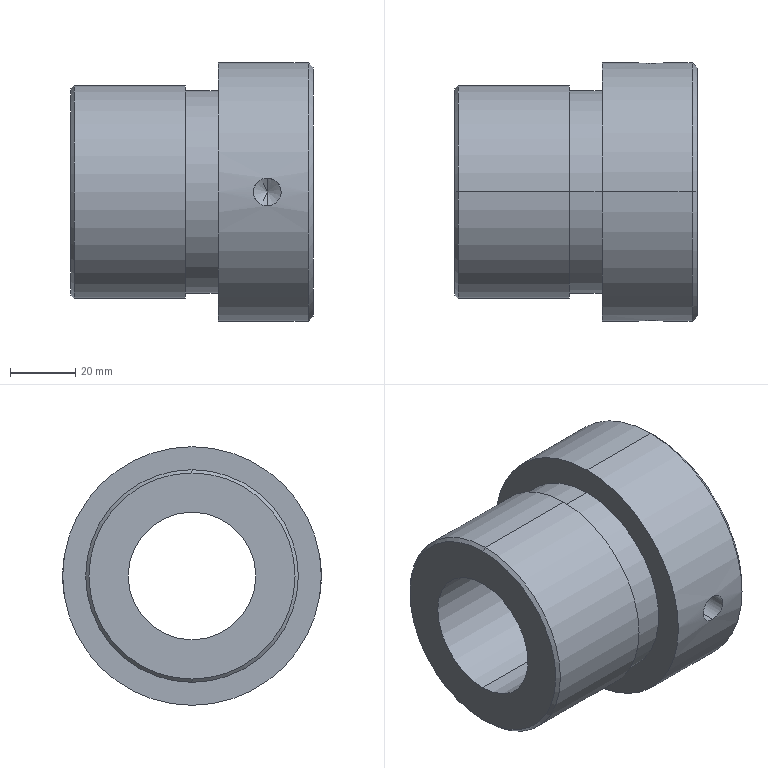Part | SolidWorks | features ICE 9, Chamfer 7, Draft 2, HoleWzd 2, Extrusion 1, Fillet 1, MirrorPattern 1, MoveFace 1 | 1 solid | 24 faces | box 74 x 79 x 79 mm | volume 198251 mm3 | cylinder 12 | cone 8 | plane 4 | commonest cylinder face diameters 8.5 x4 39 x2 62 x2 65 x2 79 x2
STEP:
#1=CARTESIAN_POINT('',(0.,0.,19.5));
#2=VERTEX_POINT('',#1);
#3=CARTESIAN_POINT('',(0.,0.,-19.5));
#4=VERTEX_POINT('',#3);
#5=CARTESIAN_POINT('',(0.,0.,0.));
#6=DIRECTION('',(1.,0.,0.));
#7=DIRECTION('',(0.,0.,-1.));
#8=AXIS2_PLACEMENT_3D('',#5,#6,#7);
#9=CIRCLE('',#8,19.5);
#10=EDGE_CURVE('',#2,#4,#9,.T.);
#11=ORIENTED_EDGE('',*,*,#10,.F.);
#12=CARTESIAN_POINT('',(74.,0.,19.5));
#13=VERTEX_POINT('',#12);
#14=CARTESIAN_POINT('',(74.,0.,19.5));
#15=DIRECTION('',(1.,0.,0.));
#16=VECTOR('',#15,1000.);
#17=LINE('',#14,#16);
#18=EDGE_CURVE('',#2,#13,#17,.T.);
#19=ORIENTED_EDGE('',*,*,#18,.T.);
#20=CARTESIAN_POINT('',(74.,0.,-19.5));
#21=VERTEX_POINT('',#20);
#22=CARTESIAN_POINT('',(74.,0.,0.));
#23=DIRECTION('',(1.,0.,0.));
#24=DIRECTION('',(0.,0.,-1.));
#25=AXIS2_PLACEMENT_3D('',#22,#23,#24);
#26=CIRCLE('',#25,19.5);
#27=EDGE_CURVE('',#13,#21,#26,.T.);
#28=ORIENTED_EDGE('',*,*,#27,.T.);
#29=CARTESIAN_POINT('',(74.,0.,-19.5));
#30=DIRECTION('',(1.,0.,0.));
#31=VECTOR('',#30,1000.);
#32=LINE('',#29,#31);
#33=EDGE_CURVE('',#4,#21,#32,.T.);
#34=ORIENTED_EDGE('',*,*,#33,.F.);
#35=EDGE_LOOP('',(#11,#19,#28,#34));
#36=FACE_OUTER_BOUND('',#35,.T.);
#37=CARTESIAN_POINT('',(74.,0.,0.));
#38=DIRECTION('',(1.,0.,0.));
#39=DIRECTION('',(0.,0.,-1.));
#40=AXIS2_PLACEMENT_3D('',#37,#38,#39);
#41=CYLINDRICAL_SURFACE('',#40,19.5);
#42=ADVANCED_FACE('',(#36),#41,.F.);
#43=CARTESIAN_POINT('',(60.,24.946,0.));
#44=VERTEX_POINT('',#43);
#45=CARTESIAN_POINT('',(60.,27.5,4.25));
#46=VERTEX_POINT('',#45);
#47=CARTESIAN_POINT('',(60.,27.5,4.25));
#48=DIRECTION('',(0.,0.515,0.8572));
#49=VECTOR('',#48,1000.);
#50=LINE('',#47,#49);
#51=EDGE_CURVE('',#44,#46,#50,.T.);
#52=ORIENTED_EDGE('',*,*,#51,.F.);
#53=CARTESIAN_POINT('',(60.,27.5,-4.25));
#54=VERTEX_POINT('',#53);
#55=CARTESIAN_POINT('',(60.,27.5,-4.25));
#56=DIRECTION('',(0.,0.515,-0.8572));
#57=VECTOR('',#56,1000.);
#58=LINE('',#55,#57);
#59=EDGE_CURVE('',#44,#54,#58,.T.);
#60=ORIENTED_EDGE('',*,*,#59,.T.);
#61=CARTESIAN_POINT('',(60.,27.5,0.));
#62=DIRECTION('',(0.,1.,0.));
#63=DIRECTION('',(0.,0.,1.));
#64=AXIS2_PLACEMENT_3D('',#61,#62,#63);
#65=CIRCLE('',#64,4.25);
#66=EDGE_CURVE('',#54,#46,#65,.T.);
#67=ORIENTED_EDGE('',*,*,#66,.T.);
#68=EDGE_LOOP('',(#52,#60,#67));
#69=FACE_OUTER_BOUND('',#68,.T.);
#70=CARTESIAN_POINT('',(60.,27.5,0.));
#71=DIRECTION('',(0.,1.,0.));
#72=DIRECTION('',(0.,0.,1.));
#73=AXIS2_PLACEMENT_3D('',#70,#71,#72);
#74=CONICAL_SURFACE('',#73,4.25,1.03);
#75=ADVANCED_FACE('',(#69),#74,.F.);
#76=ORIENTED_EDGE('',*,*,#66,.F.);
#77=CARTESIAN_POINT('',(60.,39.271,-4.25));
#78=VERTEX_POINT('',#77);
#79=CARTESIAN_POINT('',(60.,37.5,-4.25));
#80=DIRECTION('',(0.,1.,0.));
#81=VECTOR('',#80,1000.);
#82=LINE('',#79,#81);
#83=EDGE_CURVE('',#54,#78,#82,.T.);
#84=ORIENTED_EDGE('',*,*,#83,.T.);
#85=CARTESIAN_POINT('',(60.,39.271,4.25));
#86=VERTEX_POINT('',#85);
#87=CARTESIAN_POINT('',(60.,39.271,-4.25));
#88=CARTESIAN_POINT('',(59.723,39.271,-4.25));
#89=CARTESIAN_POINT('',(59.447,39.274,-4.223));
#90=CARTESIAN_POINT('',(58.898,39.285,-4.114));
#91=CARTESIAN_POINT('',(58.63,39.294,-4.033));
#92=CARTESIAN_POINT('',(58.119,39.315,-3.821));
#93=CARTESIAN_POINT('',(57.871,39.328,-3.689));
#94=CARTESIAN_POINT('',(57.407,39.356,-3.379));
#95=CARTESIAN_POINT('',(57.193,39.37,-3.203));
#96=CARTESIAN_POINT('',(56.801,39.4,-2.812));
#97=CARTESIAN_POINT('',(56.621,39.415,-2.593));
#98=CARTESIAN_POINT('',(56.313,39.443,-2.132));
#99=CARTESIAN_POINT('',(56.182,39.456,-1.888));
#100=CARTESIAN_POINT('',(55.968,39.477,-1.373));
#101=CARTESIAN_POINT('',(55.886,39.486,-1.103));
#102=CARTESIAN_POINT('',(55.778,39.497,-0.5602));
#103=CARTESIAN_POINT('',(55.75,39.5,-0.284));
#104=CARTESIAN_POINT('',(55.75,39.5,0.2777));
#105=CARTESIAN_POINT('',(55.777,39.497,0.5542));
#106=CARTESIAN_POINT('',(55.885,39.486,1.098));
#107=CARTESIAN_POINT('',(55.966,39.477,1.368));
#108=CARTESIAN_POINT('',(56.179,39.456,1.882));
#109=CARTESIAN_POINT('',(56.31,39.443,2.127));
#110=CARTESIAN_POINT('',(56.618,39.416,2.588));
#111=CARTESIAN_POINT('',(56.797,39.401,2.807));
#112=CARTESIAN_POINT('',(57.188,39.371,3.199));
#113=CARTESIAN_POINT('',(57.402,39.356,3.375));
#114=CARTESIAN_POINT('',(57.866,39.328,3.686));
#115=CARTESIAN_POINT('',(58.113,39.315,3.818));
#116=CARTESIAN_POINT('',(58.624,39.294,4.031));
#117=CARTESIAN_POINT('',(58.892,39.285,4.113));
#118=CARTESIAN_POINT('',(59.441,39.274,4.222));
#119=CARTESIAN_POINT('',(59.719,39.271,4.25));
#120=CARTESIAN_POINT('',(60.,39.271,4.25));
#121=B_SPLINE_CURVE_WITH_KNOTS('',3,(#87,#88,#89,#90,#91,#92,#93,#94,#95,#96,#97,#98,#99,#100,#101,#102,#103,#104,#105,#106,#107,#108,#109,#110,#111,#112,#113,#114,#115,#116,#117,#118,#119,#120),.UNSPECIFIED.,.F.,.F.,(4,2,2,2,2,2,2,2,2,2,2,2,2,2,2,2,4),(0.0133,0.01413,0.01496,0.01579,0.01662,0.01745,0.01828,0.01911,0.01994,0.02077,0.02161,0.02244,0.02327,0.0241,0.02493,0.02576,0.02659),.UNSPECIFIED.);
#122=EDGE_CURVE('',#78,#86,#121,.T.);
#123=ORIENTED_EDGE('',*,*,#122,.T.);
#124=CARTESIAN_POINT('',(60.,37.5,4.25));
#125=DIRECTION('',(0.,1.,0.));
#126=VECTOR('',#125,1000.);
#127=LINE('',#124,#126);
#128=EDGE_CURVE('',#46,#86,#127,.T.);
#129=ORIENTED_EDGE('',*,*,#128,.F.);
#130=EDGE_LOOP('',(#76,#84,#123,#129));
#131=FACE_OUTER_BOUND('',#130,.T.);
#132=CARTESIAN_POINT('',(60.,37.5,0.));
#133=DIRECTION('',(0.,1.,0.));
#134=DIRECTION('',(0.,0.,1.));
#135=AXIS2_PLACEMENT_3D('',#132,#133,#134);
#136=CYLINDRICAL_SURFACE('',#135,4.25);
#137=ADVANCED_FACE('',(#131),#136,.F.);
#138=CARTESIAN_POINT('',(60.,-24.946,0.));
#139=VERTEX_POINT('',#138);
#140=CARTESIAN_POINT('',(60.,-27.5,-4.25));
#141=VERTEX_POINT('',#140);
#142=CARTESIAN_POINT('',(60.,-27.5,-4.25));
#143=DIRECTION('',(0.,-0.515,-0.8572));
#144=VECTOR('',#143,1000.);
#145=LINE('',#142,#144);
#146=EDGE_CURVE('',#139,#141,#145,.T.);
#147=ORIENTED_EDGE('',*,*,#146,.F.);
#148=CARTESIAN_POINT('',(60.,-27.5,4.25));
#149=VERTEX_POINT('',#148);
#150=CARTESIAN_POINT('',(60.,-27.5,4.25));
#151=DIRECTION('',(0.,-0.515,0.8572));
#152=VECTOR('',#151,1000.);
#153=LINE('',#150,#152);
#154=EDGE_CURVE('',#139,#149,#153,.T.);
#155=ORIENTED_EDGE('',*,*,#154,.T.);
#156=CARTESIAN_POINT('',(60.,-27.5,0.));
#157=DIRECTION('',(0.,-1.,0.));
#158=DIRECTION('',(0.,0.,-1.));
#159=AXIS2_PLACEMENT_3D('',#156,#157,#158);
#160=CIRCLE('',#159,4.25);
#161=EDGE_CURVE('',#149,#141,#160,.T.);
#162=ORIENTED_EDGE('',*,*,#161,.T.);
#163=EDGE_LOOP('',(#147,#155,#162));
#164=FACE_OUTER_BOUND('',#163,.T.);
#165=CARTESIAN_POINT('',(60.,-27.5,0.));
#166=DIRECTION('',(0.,-1.,0.));
#167=DIRECTION('',(0.,0.,-1.));
#168=AXIS2_PLACEMENT_3D('',#165,#166,#167);
#169=CONICAL_SURFACE('',#168,4.25,1.03);
#170=ADVANCED_FACE('',(#164),#169,.F.);
#171=ORIENTED_EDGE('',*,*,#161,.F.);
#172=CARTESIAN_POINT('',(60.,-39.271,4.25));
#173=VERTEX_POINT('',#172);
#174=CARTESIAN_POINT('',(60.,-37.5,4.25));
#175=DIRECTION('',(0.,-1.,0.));
#176=VECTOR('',#175,1000.);
#177=LINE('',#174,#176);
#178=EDGE_CURVE('',#149,#173,#177,.T.);
#179=ORIENTED_EDGE('',*,*,#178,.T.);
#180=CARTESIAN_POINT('',(60.,-39.271,-4.25));
#181=VERTEX_POINT('',#180);
#182=CARTESIAN_POINT('',(60.,-39.271,-4.25));
#183=CARTESIAN_POINT('',(59.719,-39.271,-4.25));
#184=CARTESIAN_POINT('',(59.443,-39.274,-4.222));
#185=CARTESIAN_POINT('',(58.899,-39.285,-4.114));
#186=CARTESIAN_POINT('',(58.629,-39.294,-4.032));
#187=CARTESIAN_POINT('',(58.115,-39.315,-3.819));
#188=CARTESIAN_POINT('',(57.87,-39.328,-3.688));
#189=CARTESIAN_POINT('',(57.409,-39.355,-3.38));
#190=CARTESIAN_POINT('',(57.19,-39.371,-3.201));
#191=CARTESIAN_POINT('',(56.798,-39.401,-2.809));
#192=CARTESIAN_POINT('',(56.622,-39.415,-2.595));
#193=CARTESIAN_POINT('',(56.312,-39.443,-2.13));
#194=CARTESIAN_POINT('',(56.18,-39.456,-1.883));
#195=CARTESIAN_POINT('',(55.968,-39.477,-1.372));
#196=CARTESIAN_POINT('',(55.886,-39.486,-1.104));
#197=CARTESIAN_POINT('',(55.777,-39.497,-0.5549));
#198=CARTESIAN_POINT('',(55.75,-39.5,-0.279));
#199=CARTESIAN_POINT('',(55.75,-39.5,0.2759));
#200=CARTESIAN_POINT('',(55.778,-39.497,0.5577));
#201=CARTESIAN_POINT('',(55.886,-39.486,1.103));
#202=CARTESIAN_POINT('',(55.967,-39.477,1.368));
#203=CARTESIAN_POINT('',(56.18,-39.456,1.883));
#204=CARTESIAN_POINT('',(56.313,-39.443,2.131));
#205=CARTESIAN_POINT('',(56.62,-39.416,2.592));
#206=CARTESIAN_POINT('',(56.796,-39.401,2.806));
#207=CARTESIAN_POINT('',(57.193,-39.37,3.203));
#208=CARTESIAN_POINT('',(57.407,-39.356,3.379));
#209=CARTESIAN_POINT('',(57.867,-39.328,3.687));
#210=CARTESIAN_POINT('',(58.116,-39.315,3.82));
#211=CARTESIAN_POINT('',(58.631,-39.294,4.033));
#212=CARTESIAN_POINT('',(58.896,-39.285,4.113));
#213=CARTESIAN_POINT('',(59.441,-39.274,4.222));
#214=CARTESIAN_POINT('',(59.723,-39.271,4.25));
#215=CARTESIAN_POINT('',(60.,-39.271,4.25));
#216=B_SPLINE_CURVE_WITH_KNOTS('',3,(#182,#183,#184,#185,#186,#187,#188,#189,#190,#191,#192,#193,#194,#195,#196,#197,#198,#199,#200,#201,#202,#203,#204,#205,#206,#207,#208,#209,#210,#211,#212,#213,#214,#215),.UNSPECIFIED.,.F.,.F.,(4,2,2,2,2,2,2,2,2,2,2,2,2,2,2,2,4),(0.,0.0008311,0.001662,0.002493,0.003324,0.004155,0.004986,0.005817,0.006649,0.00748,0.008311,0.009142,0.009973,0.0108,0.01163,0.01247,0.0133),.UNSPECIFIED.);
#217=EDGE_CURVE('',#181,#173,#216,.T.);
#218=ORIENTED_EDGE('',*,*,#217,.F.);
#219=CARTESIAN_POINT('',(60.,-37.5,-4.25));
#220=DIRECTION('',(0.,-1.,0.));
#221=VECTOR('',#220,1000.);
#222=LINE('',#219,#221);
#223=EDGE_CURVE('',#141,#181,#222,.T.);
#224=ORIENTED_EDGE('',*,*,#223,.F.);
#225=EDGE_LOOP('',(#171,#179,#218,#224));
#226=FACE_OUTER_BOUND('',#225,.T.);
#227=CARTESIAN_POINT('',(60.,-37.5,0.));
#228=DIRECTION('',(0.,-1.,0.));
#229=DIRECTION('',(0.,0.,-1.));
#230=AXIS2_PLACEMENT_3D('',#227,#228,#229);
#231=CYLINDRICAL_SURFACE('',#230,4.25);
#232=ADVANCED_FACE('',(#226),#231,.F.);
#233=CARTESIAN_POINT('',(74.,0.,-38.));
#234=VERTEX_POINT('',#233);
#235=CARTESIAN_POINT('',(74.,0.,38.));
#236=VERTEX_POINT('',#235);
#237=CARTESIAN_POINT('',(74.,0.,0.));
#238=DIRECTION('',(1.,0.,0.));
#239=DIRECTION('',(0.,0.,-1.));
#240=AXIS2_PLACEMENT_3D('',#237,#238,#239);
#241=CIRCLE('',#240,38.);
#242=EDGE_CURVE('',#234,#236,#241,.T.);
#243=ORIENTED_EDGE('',*,*,#242,.F.);
#244=CARTESIAN_POINT('',(72.5,0.,-39.5));
#245=VERTEX_POINT('',#244);
#246=CARTESIAN_POINT('',(74.,0.,-38.));
#247=DIRECTION('',(-0.7071,0.,-0.7071));
#248=VECTOR('',#247,1000.);
#249=LINE('',#246,#248);
#250=EDGE_CURVE('',#234,#245,#249,.T.);
#251=ORIENTED_EDGE('',*,*,#250,.T.);
#252=CARTESIAN_POINT('',(72.5,0.,39.5));
#253=VERTEX_POINT('',#252);
#254=CARTESIAN_POINT('',(72.5,0.,0.));
#255=DIRECTION('',(-1.,0.,0.));
#256=DIRECTION('',(0.,0.,-1.));
#257=AXIS2_PLACEMENT_3D('',#254,#255,#256);
#258=CIRCLE('',#257,39.5);
#259=EDGE_CURVE('',#253,#245,#258,.T.);
#260=ORIENTED_EDGE('',*,*,#259,.F.);
#261=CARTESIAN_POINT('',(74.,0.,38.));
#262=DIRECTION('',(-0.7071,0.,0.7071));
#263=VECTOR('',#262,1000.);
#264=LINE('',#261,#263);
#265=EDGE_CURVE('',#236,#253,#264,.T.);
#266=ORIENTED_EDGE('',*,*,#265,.F.);
#267=EDGE_LOOP('',(#243,#251,#260,#266));
#268=FACE_OUTER_BOUND('',#267,.T.);
#269=CARTESIAN_POINT('',(74.,0.,0.));
#270=DIRECTION('',(-1.,0.,0.));
#271=DIRECTION('',(0.,0.,1.));
#272=AXIS2_PLACEMENT_3D('',#269,#270,#271);
#273=CONICAL_SURFACE('',#272,38.,0.7854);
#274=ADVANCED_FACE('',(#268),#273,.T.);
#275=CARTESIAN_POINT('',(0.,0.,31.5));
#276=VERTEX_POINT('',#275);
#277=CARTESIAN_POINT('',(0.,0.,-31.5));
#278=VERTEX_POINT('',#277);
#279=CARTESIAN_POINT('',(0.,0.,0.));
#280=DIRECTION('',(-1.,0.,0.));
#281=DIRECTION('',(0.,0.,-1.));
#282=AXIS2_PLACEMENT_3D('',#279,#280,#281);
#283=CIRCLE('',#282,31.5);
#284=EDGE_CURVE('',#276,#278,#283,.T.);
#285=ORIENTED_EDGE('',*,*,#284,.F.);
#286=CARTESIAN_POINT('',(1.,0.,32.5));
#287=VERTEX_POINT('',#286);
#288=CARTESIAN_POINT('',(0.,0.,31.5));
#289=DIRECTION('',(0.7071,0.,0.7071));
#290=VECTOR('',#289,1000.);
#291=LINE('',#288,#290);
#292=EDGE_CURVE('',#276,#287,#291,.T.);
#293=ORIENTED_EDGE('',*,*,#292,.T.);
#294=CARTESIAN_POINT('',(1.,0.,-32.5));
#295=VERTEX_POINT('',#294);
#296=CARTESIAN_POINT('',(1.,0.,0.));
#297=DIRECTION('',(1.,0.,0.));
#298=DIRECTION('',(0.,0.,-1.));
#299=AXIS2_PLACEMENT_3D('',#296,#297,#298);
#300=CIRCLE('',#299,32.5);
#301=EDGE_CURVE('',#295,#287,#300,.T.);
#302=ORIENTED_EDGE('',*,*,#301,.F.);
#303=CARTESIAN_POINT('',(0.,0.,-31.5));
#304=DIRECTION('',(0.7071,0.,-0.7071));
#305=VECTOR('',#304,1000.);
#306=LINE('',#303,#305);
#307=EDGE_CURVE('',#278,#295,#306,.T.);
#308=ORIENTED_EDGE('',*,*,#307,.F.);
#309=EDGE_LOOP('',(#285,#293,#302,#308));
#310=FACE_OUTER_BOUND('',#309,.T.);
#311=CARTESIAN_POINT('',(0.,0.,0.));
#312=DIRECTION('',(1.,0.,0.));
#313=DIRECTION('',(0.,0.,-1.));
#314=AXIS2_PLACEMENT_3D('',#311,#312,#313);
#315=CONICAL_SURFACE('',#314,31.5,0.7854);
#316=ADVANCED_FACE('',(#310),#315,.T.);
#317=CARTESIAN_POINT('',(35.,0.,-32.5));
#318=VERTEX_POINT('',#317);
#319=CARTESIAN_POINT('',(35.,0.,32.5));
#320=VERTEX_POINT('',#319);
#321=CARTESIAN_POINT('',(35.,0.,0.));
#322=DIRECTION('',(1.,0.,0.));
#323=DIRECTION('',(0.,0.,1.));
#324=AXIS2_PLACEMENT_3D('',#321,#322,#323);
#325=CIRCLE('',#324,32.5);
#326=EDGE_CURVE('',#318,#320,#325,.T.);
#327=ORIENTED_EDGE('',*,*,#326,.F.);
#328=CARTESIAN_POINT('',(45.,0.,-32.5));
#329=DIRECTION('',(-1.,0.,0.));
#330=VECTOR('',#329,1000.);
#331=LINE('',#328,#330);
#332=EDGE_CURVE('',#318,#295,#331,.T.);
#333=ORIENTED_EDGE('',*,*,#332,.T.);
#334=ORIENTED_EDGE('',*,*,#301,.T.);
#335=CARTESIAN_POINT('',(45.,0.,32.5));
#336=DIRECTION('',(-1.,0.,0.));
#337=VECTOR('',#336,1000.);
#338=LINE('',#335,#337);
#339=EDGE_CURVE('',#320,#287,#338,.T.);
#340=ORIENTED_EDGE('',*,*,#339,.F.);
#341=EDGE_LOOP('',(#327,#333,#334,#340));
#342=FACE_OUTER_BOUND('',#341,.T.);
#343=CARTESIAN_POINT('',(45.,0.,0.));
#344=DIRECTION('',(-1.,0.,0.));
#345=DIRECTION('',(0.,0.,1.));
#346=AXIS2_PLACEMENT_3D('',#343,#344,#345);
#347=CYLINDRICAL_SURFACE('',#346,32.5);
#348=ADVANCED_FACE('',(#342),#347,.T.);
#349=CARTESIAN_POINT('',(35.,0.,31.));
#350=VERTEX_POINT('',#349);
#351=CARTESIAN_POINT('',(35.,0.,-31.));
#352=VERTEX_POINT('',#351);
#353=CARTESIAN_POINT('',(35.,0.,0.));
#354=DIRECTION('',(-1.,0.,0.));
#355=DIRECTION('',(0.,0.,1.));
#356=AXIS2_PLACEMENT_3D('',#353,#354,#355);
#357=CIRCLE('',#356,31.);
#358=EDGE_CURVE('',#350,#352,#357,.T.);
#359=ORIENTED_EDGE('',*,*,#358,.F.);
#360=CARTESIAN_POINT('',(45.,0.,31.));
#361=VERTEX_POINT('',#360);
#362=CARTESIAN_POINT('',(35.,0.,31.));
#363=DIRECTION('',(1.,0.,0.));
#364=VECTOR('',#363,1000.);
#365=LINE('',#362,#364);
#366=EDGE_CURVE('',#350,#361,#365,.T.);
#367=ORIENTED_EDGE('',*,*,#366,.T.);
#368=CARTESIAN_POINT('',(45.,0.,-31.));
#369=VERTEX_POINT('',#368);
#370=CARTESIAN_POINT('',(45.,0.,0.));
#371=DIRECTION('',(-1.,0.,0.));
#372=DIRECTION('',(0.,0.,1.));
#373=AXIS2_PLACEMENT_3D('',#370,#371,#372);
#374=CIRCLE('',#373,31.);
#375=EDGE_CURVE('',#361,#369,#374,.T.);
#376=ORIENTED_EDGE('',*,*,#375,.T.);
#377=CARTESIAN_POINT('',(35.,0.,-31.));
#378=DIRECTION('',(1.,0.,0.));
#379=VECTOR('',#378,1000.);
#380=LINE('',#377,#379);
#381=EDGE_CURVE('',#352,#369,#380,.T.);
#382=ORIENTED_EDGE('',*,*,#381,.F.);
#383=EDGE_LOOP('',(#359,#367,#376,#382));
#384=FACE_OUTER_BOUND('',#383,.T.);
#385=CARTESIAN_POINT('',(35.,0.,0.));
#386=DIRECTION('',(1.,0.,0.));
#387=DIRECTION('',(0.,0.,-1.));
#388=AXIS2_PLACEMENT_3D('',#385,#386,#387);
#389=CYLINDRICAL_SURFACE('',#388,31.);
#390=ADVANCED_FACE('',(#384),#389,.T.);
#391=CARTESIAN_POINT('',(60.,39.271,4.25));
#392=CARTESIAN_POINT('',(60.281,39.271,4.25));
#393=CARTESIAN_POINT('',(60.557,39.274,4.222));
#394=CARTESIAN_POINT('',(61.101,39.285,4.114));
#395=CARTESIAN_POINT('',(61.371,39.294,4.032));
#396=CARTESIAN_POINT('',(61.885,39.315,3.819));
#397=CARTESIAN_POINT('',(62.13,39.328,3.688));
#398=CARTESIAN_POINT('',(62.591,39.355,3.38));
#399=CARTESIAN_POINT('',(62.81,39.371,3.201));
#400=CARTESIAN_POINT('',(63.202,39.401,2.809));
#401=CARTESIAN_POINT('',(63.378,39.415,2.595));
#402=CARTESIAN_POINT('',(63.688,39.443,2.13));
#403=CARTESIAN_POINT('',(63.82,39.456,1.883));
#404=CARTESIAN_POINT('',(64.032,39.477,1.372));
#405=CARTESIAN_POINT('',(64.114,39.486,1.104));
#406=CARTESIAN_POINT('',(64.223,39.497,0.5549));
#407=CARTESIAN_POINT('',(64.25,39.5,0.279));
#408=CARTESIAN_POINT('',(64.25,39.5,-0.2759));
#409=CARTESIAN_POINT('',(64.222,39.497,-0.5577));
#410=CARTESIAN_POINT('',(64.114,39.486,-1.103));
#411=CARTESIAN_POINT('',(64.033,39.477,-1.368));
#412=CARTESIAN_POINT('',(63.82,39.456,-1.883));
#413=CARTESIAN_POINT('',(63.687,39.443,-2.131));
#414=CARTESIAN_POINT('',(63.38,39.416,-2.592));
#415=CARTESIAN_POINT('',(63.204,39.401,-2.806));
#416=CARTESIAN_POINT('',(62.807,39.37,-3.203));
#417=CARTESIAN_POINT('',(62.593,39.356,-3.379));
#418=CARTESIAN_POINT('',(62.133,39.328,-3.687));
#419=CARTESIAN_POINT('',(61.884,39.315,-3.82));
#420=CARTESIAN_POINT('',(61.369,39.294,-4.033));
#421=CARTESIAN_POINT('',(61.104,39.285,-4.113));
#422=CARTESIAN_POINT('',(60.559,39.274,-4.222));
#423=CARTESIAN_POINT('',(60.277,39.271,-4.25));
#424=CARTESIAN_POINT('',(60.,39.271,-4.25));
#425=B_SPLINE_CURVE_WITH_KNOTS('',3,(#391,#392,#393,#394,#395,#396,#397,#398,#399,#400,#401,#402,#403,#404,#405,#406,#407,#408,#409,#410,#411,#412,#413,#414,#415,#416,#417,#418,#419,#420,#421,#422,#423,#424),.UNSPECIFIED.,.F.,.F.,(4,2,2,2,2,2,2,2,2,2,2,2,2,2,2,2,4),(0.,0.0008311,0.001662,0.002493,0.003324,0.004155,0.004986,0.005817,0.006649,0.00748,0.008311,0.009142,0.009973,0.0108,0.01163,0.01247,0.0133),.UNSPECIFIED.);
#426=EDGE_CURVE('',#86,#78,#425,.T.);
#427=ORIENTED_EDGE('',*,*,#426,.F.);
#428=ORIENTED_EDGE('',*,*,#122,.F.);
#429=EDGE_LOOP('',(#427,#428));
#430=FACE_BOUND('',#429,.T.);
#431=ORIENTED_EDGE('',*,*,#259,.T.);
#432=CARTESIAN_POINT('',(45.,0.,-39.5));
#433=VERTEX_POINT('',#432);
#434=CARTESIAN_POINT('',(144.,0.,-39.5));
#435=DIRECTION('',(-1.,0.,0.));
#436=VECTOR('',#435,1000.);
#437=LINE('',#434,#436);
#438=EDGE_CURVE('',#245,#433,#437,.T.);
#439=ORIENTED_EDGE('',*,*,#438,.T.);
#440=CARTESIAN_POINT('',(45.,0.,39.5));
#441=VERTEX_POINT('',#440);
#442=CARTESIAN_POINT('',(45.,0.,0.));
#443=DIRECTION('',(-1.,0.,0.));
#444=DIRECTION('',(0.,0.,1.));
#445=AXIS2_PLACEMENT_3D('',#442,#443,#444);
#446=CIRCLE('',#445,39.5);
#447=EDGE_CURVE('',#441,#433,#446,.T.);
#448=ORIENTED_EDGE('',*,*,#447,.F.);
#449=CARTESIAN_POINT('',(144.,0.,39.5));
#450=DIRECTION('',(-1.,0.,0.));
#451=VECTOR('',#450,1000.);
#452=LINE('',#449,#451);
#453=EDGE_CURVE('',#253,#441,#452,.T.);
#454=ORIENTED_EDGE('',*,*,#453,.F.);
#455=EDGE_LOOP('',(#431,#439,#448,#454));
#456=FACE_OUTER_BOUND('',#455,.T.);
#457=CARTESIAN_POINT('',(144.,0.,0.));
#458=DIRECTION('',(-1.,0.,0.));
#459=DIRECTION('',(0.,0.,1.));
#460=AXIS2_PLACEMENT_3D('',#457,#458,#459);
#461=CYLINDRICAL_SURFACE('',#460,39.5);
#462=ADVANCED_FACE('',(#430,#456),#461,.T.);
#463=ORIENTED_EDGE('',*,*,#438,.F.);
#464=CARTESIAN_POINT('',(72.5,0.,0.));
#465=DIRECTION('',(-1.,0.,0.));
#466=DIRECTION('',(0.,0.,-1.));
#467=AXIS2_PLACEMENT_3D('',#464,#465,#466);
#468=CIRCLE('',#467,39.5);
#469=EDGE_CURVE('',#245,#253,#468,.T.);
#470=ORIENTED_EDGE('',*,*,#469,.T.);
#471=ORIENTED_EDGE('',*,*,#453,.T.);
#472=CARTESIAN_POINT('',(45.,0.,0.));
#473=DIRECTION('',(-1.,0.,0.));
#474=DIRECTION('',(0.,0.,1.));
#475=AXIS2_PLACEMENT_3D('',#472,#473,#474);
#476=CIRCLE('',#475,39.5);
#477=EDGE_CURVE('',#433,#441,#476,.T.);
#478=ORIENTED_EDGE('',*,*,#477,.F.);
#479=EDGE_LOOP('',(#463,#470,#471,#478));
#480=FACE_OUTER_BOUND('',#479,.T.);
#481=ORIENTED_EDGE('',*,*,#217,.T.);
#482=CARTESIAN_POINT('',(60.,-39.271,4.25));
#483=CARTESIAN_POINT('',(60.277,-39.271,4.25));
#484=CARTESIAN_POINT('',(60.553,-39.274,4.223));
#485=CARTESIAN_POINT('',(61.102,-39.285,4.114));
#486=CARTESIAN_POINT('',(61.37,-39.294,4.033));
#487=CARTESIAN_POINT('',(61.881,-39.315,3.821));
#488=CARTESIAN_POINT('',(62.129,-39.328,3.689));
#489=CARTESIAN_POINT('',(62.593,-39.356,3.379));
#490=CARTESIAN_POINT('',(62.807,-39.37,3.203));
#491=CARTESIAN_POINT('',(63.199,-39.4,2.812));
#492=CARTESIAN_POINT('',(63.379,-39.415,2.593));
#493=CARTESIAN_POINT('',(63.687,-39.443,2.132));
#494=CARTESIAN_POINT('',(63.818,-39.456,1.888));
#495=CARTESIAN_POINT('',(64.032,-39.477,1.373));
#496=CARTESIAN_POINT('',(64.114,-39.486,1.103));
#497=CARTESIAN_POINT('',(64.222,-39.497,0.5602));
#498=CARTESIAN_POINT('',(64.25,-39.5,0.284));
#499=CARTESIAN_POINT('',(64.25,-39.5,-0.2777));
#500=CARTESIAN_POINT('',(64.223,-39.497,-0.5542));
#501=CARTESIAN_POINT('',(64.115,-39.486,-1.098));
#502=CARTESIAN_POINT('',(64.034,-39.477,-1.368));
#503=CARTESIAN_POINT('',(63.821,-39.456,-1.882));
#504=CARTESIAN_POINT('',(63.69,-39.443,-2.127));
#505=CARTESIAN_POINT('',(63.382,-39.416,-2.588));
#506=CARTESIAN_POINT('',(63.203,-39.401,-2.807));
#507=CARTESIAN_POINT('',(62.812,-39.371,-3.199));
#508=CARTESIAN_POINT('',(62.598,-39.356,-3.375));
#509=CARTESIAN_POINT('',(62.134,-39.328,-3.686));
#510=CARTESIAN_POINT('',(61.887,-39.315,-3.818));
#511=CARTESIAN_POINT('',(61.376,-39.294,-4.031));
#512=CARTESIAN_POINT('',(61.108,-39.285,-4.113));
#513=CARTESIAN_POINT('',(60.559,-39.274,-4.222));
#514=CARTESIAN_POINT('',(60.281,-39.271,-4.25));
#515=CARTESIAN_POINT('',(60.,-39.271,-4.25));
#516=B_SPLINE_CURVE_WITH_KNOTS('',3,(#482,#483,#484,#485,#486,#487,#488,#489,#490,#491,#492,#493,#494,#495,#496,#497,#498,#499,#500,#501,#502,#503,#504,#505,#506,#507,#508,#509,#510,#511,#512,#513,#514,#515),.UNSPECIFIED.,.F.,.F.,(4,2,2,2,2,2,2,2,2,2,2,2,2,2,2,2,4),(0.0133,0.01413,0.01496,0.01579,0.01662,0.01745,0.01828,0.01911,0.01994,0.02077,0.02161,0.02244,0.02327,0.0241,0.02493,0.02576,0.02659),.UNSPECIFIED.);
#517=EDGE_CURVE('',#173,#181,#516,.T.);
#518=ORIENTED_EDGE('',*,*,#517,.T.);
#519=EDGE_LOOP('',(#481,#518));
#520=FACE_BOUND('',#519,.T.);
#521=CARTESIAN_POINT('',(144.,0.,0.));
#522=DIRECTION('',(-1.,0.,0.));
#523=DIRECTION('',(0.,0.,1.));
#524=AXIS2_PLACEMENT_3D('',#521,#522,#523);
#525=CYLINDRICAL_SURFACE('',#524,39.5);
#526=ADVANCED_FACE('',(#480,#520),#525,.T.);
#527=CARTESIAN_POINT('',(74.,0.,0.));
#528=DIRECTION('',(1.,0.,0.));
#529=DIRECTION('',(0.,0.,-1.));
#530=AXIS2_PLACEMENT_3D('',#527,#528,#529);
#531=CIRCLE('',#530,19.5);
#532=EDGE_CURVE('',#21,#13,#531,.T.);
#533=ORIENTED_EDGE('',*,*,#532,.F.);
#534=ORIENTED_EDGE('',*,*,#27,.F.);
#535=EDGE_LOOP('',(#533,#534));
#536=FACE_BOUND('',#535,.T.);
#537=CARTESIAN_POINT('',(74.,0.,0.));
#538=DIRECTION('',(1.,0.,0.));
#539=DIRECTION('',(0.,0.,-1.));
#540=AXIS2_PLACEMENT_3D('',#537,#538,#539);
#541=CIRCLE('',#540,38.);
#542=EDGE_CURVE('',#236,#234,#541,.T.);
#543=ORIENTED_EDGE('',*,*,#542,.T.);
#544=ORIENTED_EDGE('',*,*,#242,.T.);
#545=EDGE_LOOP('',(#543,#544));
#546=FACE_OUTER_BOUND('',#545,.T.);
#547=CARTESIAN_POINT('',(74.,0.,0.));
#548=DIRECTION('',(1.,0.,0.));
#549=DIRECTION('',(0.,0.,-1.));
#550=AXIS2_PLACEMENT_3D('',#547,#548,#549);
#551=PLANE('',#550);
#552=ADVANCED_FACE('',(#536,#546),#551,.T.);
#553=ORIENTED_EDGE('',*,*,#447,.T.);
#554=ORIENTED_EDGE('',*,*,#477,.T.);
#555=EDGE_LOOP('',(#553,#554));
#556=FACE_OUTER_BOUND('',#555,.T.);
#557=CARTESIAN_POINT('',(45.,0.,0.));
#558=DIRECTION('',(-1.,0.,0.));
#559=DIRECTION('',(0.,0.,1.));
#560=AXIS2_PLACEMENT_3D('',#557,#558,#559);
#561=CIRCLE('',#560,31.);
#562=EDGE_CURVE('',#369,#361,#561,.T.);
#563=ORIENTED_EDGE('',*,*,#562,.F.);
#564=ORIENTED_EDGE('',*,*,#375,.F.);
#565=EDGE_LOOP('',(#563,#564));
#566=FACE_BOUND('',#565,.T.);
#567=CARTESIAN_POINT('',(45.,0.,0.));
#568=DIRECTION('',(-1.,0.,0.));
#569=DIRECTION('',(0.,0.,1.));
#570=AXIS2_PLACEMENT_3D('',#567,#568,#569);
#571=PLANE('',#570);
#572=ADVANCED_FACE('',(#556,#566),#571,.T.);
#573=CARTESIAN_POINT('',(35.,0.,0.));
#574=DIRECTION('',(1.,0.,0.));
#575=DIRECTION('',(0.,0.,1.));
#576=AXIS2_PLACEMENT_3D('',#573,#574,#575);
#577=CIRCLE('',#576,32.5);
#578=EDGE_CURVE('',#320,#318,#577,.T.);
#579=ORIENTED_EDGE('',*,*,#578,.T.);
#580=ORIENTED_EDGE('',*,*,#326,.T.);
#581=EDGE_LOOP('',(#579,#580));
#582=FACE_OUTER_BOUND('',#581,.T.);
#583=CARTESIAN_POINT('',(35.,0.,0.));
#584=DIRECTION('',(-1.,0.,0.));
#585=DIRECTION('',(0.,0.,1.));
#586=AXIS2_PLACEMENT_3D('',#583,#584,#585);
#587=CIRCLE('',#586,31.);
#588=EDGE_CURVE('',#352,#350,#587,.T.);
#589=ORIENTED_EDGE('',*,*,#588,.T.);
#590=ORIENTED_EDGE('',*,*,#358,.T.);
#591=EDGE_LOOP('',(#589,#590));
#592=FACE_BOUND('',#591,.T.);
#593=CARTESIAN_POINT('',(35.,0.,0.));
#594=DIRECTION('',(-1.,0.,0.));
#595=DIRECTION('',(0.,0.,1.));
#596=AXIS2_PLACEMENT_3D('',#593,#594,#595);
#597=PLANE('',#596);
#598=ADVANCED_FACE('',(#582,#592),#597,.F.);
#599=ORIENTED_EDGE('',*,*,#366,.F.);
#600=ORIENTED_EDGE('',*,*,#588,.F.);
#601=ORIENTED_EDGE('',*,*,#381,.T.);
#602=ORIENTED_EDGE('',*,*,#562,.T.);
#603=EDGE_LOOP('',(#599,#600,#601,#602));
#604=FACE_OUTER_BOUND('',#603,.T.);
#605=CARTESIAN_POINT('',(35.,0.,0.));
#606=DIRECTION('',(1.,0.,0.));
#607=DIRECTION('',(0.,0.,-1.));
#608=AXIS2_PLACEMENT_3D('',#605,#606,#607);
#609=CYLINDRICAL_SURFACE('',#608,31.);
#610=ADVANCED_FACE('',(#604),#609,.T.);
#611=CARTESIAN_POINT('',(0.,0.,0.));
#612=DIRECTION('',(1.,0.,0.));
#613=DIRECTION('',(0.,0.,-1.));
#614=AXIS2_PLACEMENT_3D('',#611,#612,#613);
#615=CIRCLE('',#614,19.5);
#616=EDGE_CURVE('',#4,#2,#615,.T.);
#617=ORIENTED_EDGE('',*,*,#616,.T.);
#618=ORIENTED_EDGE('',*,*,#10,.T.);
#619=EDGE_LOOP('',(#617,#618));
#620=FACE_BOUND('',#619,.T.);
#621=CARTESIAN_POINT('',(0.,0.,0.));
#622=DIRECTION('',(-1.,0.,0.));
#623=DIRECTION('',(0.,0.,-1.));
#624=AXIS2_PLACEMENT_3D('',#621,#622,#623);
#625=CIRCLE('',#624,31.5);
#626=EDGE_CURVE('',#278,#276,#625,.T.);
#627=ORIENTED_EDGE('',*,*,#626,.T.);
#628=ORIENTED_EDGE('',*,*,#284,.T.);
#629=EDGE_LOOP('',(#627,#628));
#630=FACE_OUTER_BOUND('',#629,.T.);
#631=CARTESIAN_POINT('',(0.,0.,0.));
#632=DIRECTION('',(1.,0.,0.));
#633=DIRECTION('',(0.,0.,-1.));
#634=AXIS2_PLACEMENT_3D('',#631,#632,#633);
#635=PLANE('',#634);
#636=ADVANCED_FACE('',(#620,#630),#635,.F.);
#637=ORIENTED_EDGE('',*,*,#332,.F.);
#638=ORIENTED_EDGE('',*,*,#578,.F.);
#639=ORIENTED_EDGE('',*,*,#339,.T.);
#640=CARTESIAN_POINT('',(1.,0.,0.));
#641=DIRECTION('',(1.,0.,0.));
#642=DIRECTION('',(0.,0.,-1.));
#643=AXIS2_PLACEMENT_3D('',#640,#641,#642);
#644=CIRCLE('',#643,32.5);
#645=EDGE_CURVE('',#287,#295,#644,.T.);
#646=ORIENTED_EDGE('',*,*,#645,.T.);
#647=EDGE_LOOP('',(#637,#638,#639,#646));
#648=FACE_OUTER_BOUND('',#647,.T.);
#649=CARTESIAN_POINT('',(45.,0.,0.));
#650=DIRECTION('',(-1.,0.,0.));
#651=DIRECTION('',(0.,0.,1.));
#652=AXIS2_PLACEMENT_3D('',#649,#650,#651);
#653=CYLINDRICAL_SURFACE('',#652,32.5);
#654=ADVANCED_FACE('',(#648),#653,.T.);
#655=ORIENTED_EDGE('',*,*,#292,.F.);
#656=ORIENTED_EDGE('',*,*,#626,.F.);
#657=ORIENTED_EDGE('',*,*,#307,.T.);
#658=ORIENTED_EDGE('',*,*,#645,.F.);
#659=EDGE_LOOP('',(#655,#656,#657,#658));
#660=FACE_OUTER_BOUND('',#659,.T.);
#661=CARTESIAN_POINT('',(0.,0.,0.));
#662=DIRECTION('',(1.,0.,0.));
#663=DIRECTION('',(0.,0.,-1.));
#664=AXIS2_PLACEMENT_3D('',#661,#662,#663);
#665=CONICAL_SURFACE('',#664,31.5,0.7854);
#666=ADVANCED_FACE('',(#660),#665,.T.);
#667=ORIENTED_EDGE('',*,*,#250,.F.);
#668=ORIENTED_EDGE('',*,*,#542,.F.);
#669=ORIENTED_EDGE('',*,*,#265,.T.);
#670=ORIENTED_EDGE('',*,*,#469,.F.);
#671=EDGE_LOOP('',(#667,#668,#669,#670));
#672=FACE_OUTER_BOUND('',#671,.T.);
#673=CARTESIAN_POINT('',(74.,0.,0.));
#674=DIRECTION('',(-1.,0.,0.));
#675=DIRECTION('',(0.,0.,1.));
#676=AXIS2_PLACEMENT_3D('',#673,#674,#675);
#677=CONICAL_SURFACE('',#676,38.,0.7854);
#678=ADVANCED_FACE('',(#672),#677,.T.);
#679=ORIENTED_EDGE('',*,*,#178,.F.);
#680=CARTESIAN_POINT('',(60.,-27.5,0.));
#681=DIRECTION('',(0.,-1.,0.));
#682=DIRECTION('',(0.,0.,-1.));
#683=AXIS2_PLACEMENT_3D('',#680,#681,#682);
#684=CIRCLE('',#683,4.25);
#685=EDGE_CURVE('',#141,#149,#684,.T.);
#686=ORIENTED_EDGE('',*,*,#685,.F.);
#687=ORIENTED_EDGE('',*,*,#223,.T.);
#688=ORIENTED_EDGE('',*,*,#517,.F.);
#689=EDGE_LOOP('',(#679,#686,#687,#688));
#690=FACE_OUTER_BOUND('',#689,.T.);
#691=CARTESIAN_POINT('',(60.,-37.5,0.));
#692=DIRECTION('',(0.,-1.,0.));
#693=DIRECTION('',(0.,0.,-1.));
#694=AXIS2_PLACEMENT_3D('',#691,#692,#693);
#695=CYLINDRICAL_SURFACE('',#694,4.25);
#696=ADVANCED_FACE('',(#690),#695,.F.);
#697=ORIENTED_EDGE('',*,*,#154,.F.);
#698=ORIENTED_EDGE('',*,*,#146,.T.);
#699=ORIENTED_EDGE('',*,*,#685,.T.);
#700=EDGE_LOOP('',(#697,#698,#699));
#701=FACE_OUTER_BOUND('',#700,.T.);
#702=CARTESIAN_POINT('',(60.,-27.5,0.));
#703=DIRECTION('',(0.,-1.,0.));
#704=DIRECTION('',(0.,0.,-1.));
#705=AXIS2_PLACEMENT_3D('',#702,#703,#704);
#706=CONICAL_SURFACE('',#705,4.25,1.03);
#707=ADVANCED_FACE('',(#701),#706,.F.);
#708=ORIENTED_EDGE('',*,*,#83,.F.);
#709=CARTESIAN_POINT('',(60.,27.5,0.));
#710=DIRECTION('',(0.,1.,0.));
#711=DIRECTION('',(0.,0.,1.));
#712=AXIS2_PLACEMENT_3D('',#709,#710,#711);
#713=CIRCLE('',#712,4.25);
#714=EDGE_CURVE('',#46,#54,#713,.T.);
#715=ORIENTED_EDGE('',*,*,#714,.F.);
#716=ORIENTED_EDGE('',*,*,#128,.T.);
#717=ORIENTED_EDGE('',*,*,#426,.T.);
#718=EDGE_LOOP('',(#708,#715,#716,#717));
#719=FACE_OUTER_BOUND('',#718,.T.);
#720=CARTESIAN_POINT('',(60.,37.5,0.));
#721=DIRECTION('',(0.,1.,0.));
#722=DIRECTION('',(0.,0.,1.));
#723=AXIS2_PLACEMENT_3D('',#720,#721,#722);
#724=CYLINDRICAL_SURFACE('',#723,4.25);
#725=ADVANCED_FACE('',(#719),#724,.F.);
#726=ORIENTED_EDGE('',*,*,#59,.F.);
#727=ORIENTED_EDGE('',*,*,#51,.T.);
#728=ORIENTED_EDGE('',*,*,#714,.T.);
#729=EDGE_LOOP('',(#726,#727,#728));
#730=FACE_OUTER_BOUND('',#729,.T.);
#731=CARTESIAN_POINT('',(60.,27.5,0.));
#732=DIRECTION('',(0.,1.,0.));
#733=DIRECTION('',(0.,0.,1.));
#734=AXIS2_PLACEMENT_3D('',#731,#732,#733);
#735=CONICAL_SURFACE('',#734,4.25,1.03);
#736=ADVANCED_FACE('',(#730),#735,.F.);
#737=ORIENTED_EDGE('',*,*,#18,.F.);
#738=ORIENTED_EDGE('',*,*,#616,.F.);
#739=ORIENTED_EDGE('',*,*,#33,.T.);
#740=ORIENTED_EDGE('',*,*,#532,.T.);
#741=EDGE_LOOP('',(#737,#738,#739,#740));
#742=FACE_OUTER_BOUND('',#741,.T.);
#743=CARTESIAN_POINT('',(74.,0.,0.));
#744=DIRECTION('',(1.,0.,0.));
#745=DIRECTION('',(0.,0.,-1.));
#746=AXIS2_PLACEMENT_3D('',#743,#744,#745);
#747=CYLINDRICAL_SURFACE('',#746,19.5);
#748=ADVANCED_FACE('',(#742),#747,.F.);
#749=CLOSED_SHELL('',(#42,#75,#137,#170,#232,#274,#316,#348,#390,#462,#526,#552,#572,#598,#610,#636,#654,#666,#678,#696,#707,#725,#736,#748));
#750=MANIFOLD_SOLID_BREP('',#749);
#751=CARTESIAN_POINT('',(0.,0.,0.));
#752=DIRECTION('',(0.,0.,1.));
#753=DIRECTION('',(1.,0.,0.));
#754=AXIS2_PLACEMENT_3D('',#751,#752,#753);
#755=(LENGTH_UNIT()NAMED_UNIT(*)SI_UNIT(.MILLI.,.METRE.));
#756=UNCERTAINTY_MEASURE_WITH_UNIT(LENGTH_MEASURE(0.00001),#755,'','');
#757=(NAMED_UNIT(*)PLANE_ANGLE_UNIT()SI_UNIT($,.RADIAN.));
#758=(NAMED_UNIT(*)SI_UNIT($,.STERADIAN.)SOLID_ANGLE_UNIT());
#759=(GEOMETRIC_REPRESENTATION_CONTEXT(3)GLOBAL_UNCERTAINTY_ASSIGNED_CONTEXT((#756))GLOBAL_UNIT_ASSIGNED_CONTEXT((#755,#757,#758))REPRESENTATION_CONTEXT('',''));
#760=ADVANCED_BREP_SHAPE_REPRESENTATION('',(#750,#754),#759);